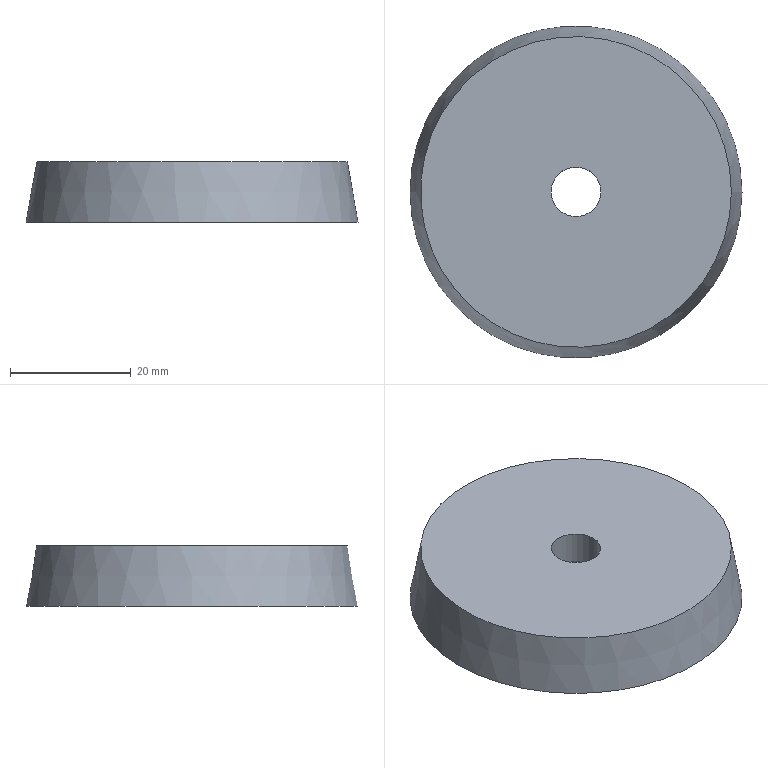Part | NX | features DATUM_CSYS 3, SKETCH 2, ASSOCIATIVE_INTERSECTION 1, EXTRUDE 1, SWP104 1 | 1 solid | 5 faces | box 55 x 55 x 10 mm | volume 21401 mm3 | cone 2 | plane 2 | cylinder 1 | commonest cylinder face diameters 8.2 x1
STEP:
#1=CARTESIAN_POINT('',(25.737,0.,10.));
#2=VERTEX_POINT('',#1);
#3=CARTESIAN_POINT('',(0.,0.,10.));
#4=DIRECTION('',(0.,0.,1.));
#5=DIRECTION('',(1.,0.,0.));
#6=AXIS2_PLACEMENT_3D('',#3,#4,#5);
#7=CIRCLE('',#6,25.737);
#8=EDGE_CURVE('',#2,#2,#7,.T.);
#9=ORIENTED_EDGE('',*,*,#8,.F.);
#10=EDGE_LOOP('',(#9));
#11=FACE_BOUND('',#10,.T.);
#12=CARTESIAN_POINT('',(27.5,0.,0.));
#13=VERTEX_POINT('',#12);
#14=CARTESIAN_POINT('',(0.,0.,0.));
#15=DIRECTION('',(0.,0.,1.));
#16=DIRECTION('',(1.,0.,0.));
#17=AXIS2_PLACEMENT_3D('',#14,#15,#16);
#18=CIRCLE('',#17,27.5);
#19=EDGE_CURVE('',#13,#13,#18,.T.);
#20=ORIENTED_EDGE('',*,*,#19,.T.);
#21=EDGE_LOOP('',(#20));
#22=FACE_BOUND('',#21,.T.);
#23=CARTESIAN_POINT('',(0.,0.,0.));
#24=DIRECTION('',(0.,0.,-1.));
#25=DIRECTION('',(1.,0.,0.));
#26=AXIS2_PLACEMENT_3D('',#23,#24,#25);
#27=CONICAL_SURFACE('',#26,27.5,0.1745);
#28=ADVANCED_FACE('',(#11,#22),#27,.T.);
#29=CARTESIAN_POINT('',(4.1,0.,10.));
#30=VERTEX_POINT('',#29);
#31=CARTESIAN_POINT('',(0.,0.,10.));
#32=DIRECTION('',(0.,0.,1.));
#33=DIRECTION('',(1.,0.,0.));
#34=AXIS2_PLACEMENT_3D('',#31,#32,#33);
#35=CIRCLE('',#34,4.1);
#36=EDGE_CURVE('',#30,#30,#35,.T.);
#37=ORIENTED_EDGE('',*,*,#36,.F.);
#38=EDGE_LOOP('',(#37));
#39=FACE_BOUND('',#38,.T.);
#40=ORIENTED_EDGE('',*,*,#8,.T.);
#41=EDGE_LOOP('',(#40));
#42=FACE_BOUND('',#41,.T.);
#43=CARTESIAN_POINT('',(0.,0.,10.));
#44=DIRECTION('',(0.,0.,1.));
#45=DIRECTION('',(1.,0.,0.));
#46=AXIS2_PLACEMENT_3D('',#43,#44,#45);
#47=PLANE('',#46);
#48=ADVANCED_FACE('',(#39,#42),#47,.T.);
#49=CARTESIAN_POINT('',(8.5,0.,0.));
#50=VERTEX_POINT('',#49);
#51=CARTESIAN_POINT('',(0.,0.,0.));
#52=DIRECTION('',(0.,0.,1.));
#53=DIRECTION('',(1.,0.,0.));
#54=AXIS2_PLACEMENT_3D('',#51,#52,#53);
#55=CIRCLE('',#54,8.5);
#56=EDGE_CURVE('',#50,#50,#55,.T.);
#57=ORIENTED_EDGE('',*,*,#56,.T.);
#58=EDGE_LOOP('',(#57));
#59=FACE_BOUND('',#58,.T.);
#60=ORIENTED_EDGE('',*,*,#19,.F.);
#61=EDGE_LOOP('',(#60));
#62=FACE_BOUND('',#61,.T.);
#63=CARTESIAN_POINT('',(0.,0.,0.));
#64=DIRECTION('',(0.,0.,1.));
#65=DIRECTION('',(1.,0.,0.));
#66=AXIS2_PLACEMENT_3D('',#63,#64,#65);
#67=PLANE('',#66);
#68=ADVANCED_FACE('',(#59,#62),#67,.F.);
#69=ORIENTED_EDGE('',*,*,#56,.F.);
#70=EDGE_LOOP('',(#69));
#71=FACE_BOUND('',#70,.T.);
#72=CARTESIAN_POINT('',(4.1,0.,4.4));
#73=VERTEX_POINT('',#72);
#74=CARTESIAN_POINT('',(0.,0.,4.4));
#75=DIRECTION('',(0.,0.,1.));
#76=DIRECTION('',(1.,0.,0.));
#77=AXIS2_PLACEMENT_3D('',#74,#75,#76);
#78=CIRCLE('',#77,4.1);
#79=EDGE_CURVE('',#73,#73,#78,.F.);
#80=ORIENTED_EDGE('',*,*,#79,.F.);
#81=EDGE_LOOP('',(#80));
#82=FACE_BOUND('',#81,.T.);
#83=CARTESIAN_POINT('',(0.,0.,4.4));
#84=DIRECTION('',(0.,0.,-1.));
#85=DIRECTION('',(-1.,0.,0.));
#86=AXIS2_PLACEMENT_3D('',#83,#84,#85);
#87=CONICAL_SURFACE('',#86,4.1,0.7854);
#88=ADVANCED_FACE('',(#71,#82),#87,.F.);
#89=ORIENTED_EDGE('',*,*,#79,.T.);
#90=EDGE_LOOP('',(#89));
#91=FACE_BOUND('',#90,.T.);
#92=ORIENTED_EDGE('',*,*,#36,.T.);
#93=EDGE_LOOP('',(#92));
#94=FACE_BOUND('',#93,.T.);
#95=CARTESIAN_POINT('',(0.,0.,0.));
#96=DIRECTION('',(0.,0.,1.));
#97=DIRECTION('',(1.,0.,0.));
#98=AXIS2_PLACEMENT_3D('',#95,#96,#97);
#99=CYLINDRICAL_SURFACE('',#98,4.1);
#100=ADVANCED_FACE('',(#91,#94),#99,.F.);
#101=CLOSED_SHELL('',(#28,#48,#68,#88,#100));
#102=MANIFOLD_SOLID_BREP('',#101);
#103=(LENGTH_UNIT()NAMED_UNIT(*)SI_UNIT(.MILLI.,.METRE.));
#104=UNCERTAINTY_MEASURE_WITH_UNIT(LENGTH_MEASURE(0.00001),#103,'','');
#105=(NAMED_UNIT(*)PLANE_ANGLE_UNIT()SI_UNIT($,.RADIAN.));
#106=(NAMED_UNIT(*)SI_UNIT($,.STERADIAN.)SOLID_ANGLE_UNIT());
#107=(GEOMETRIC_REPRESENTATION_CONTEXT(3)GLOBAL_UNCERTAINTY_ASSIGNED_CONTEXT((#104))GLOBAL_UNIT_ASSIGNED_CONTEXT((#103,#105,#106))REPRESENTATION_CONTEXT('',''));
#108=ADVANCED_BREP_SHAPE_REPRESENTATION('',(#102),#107);